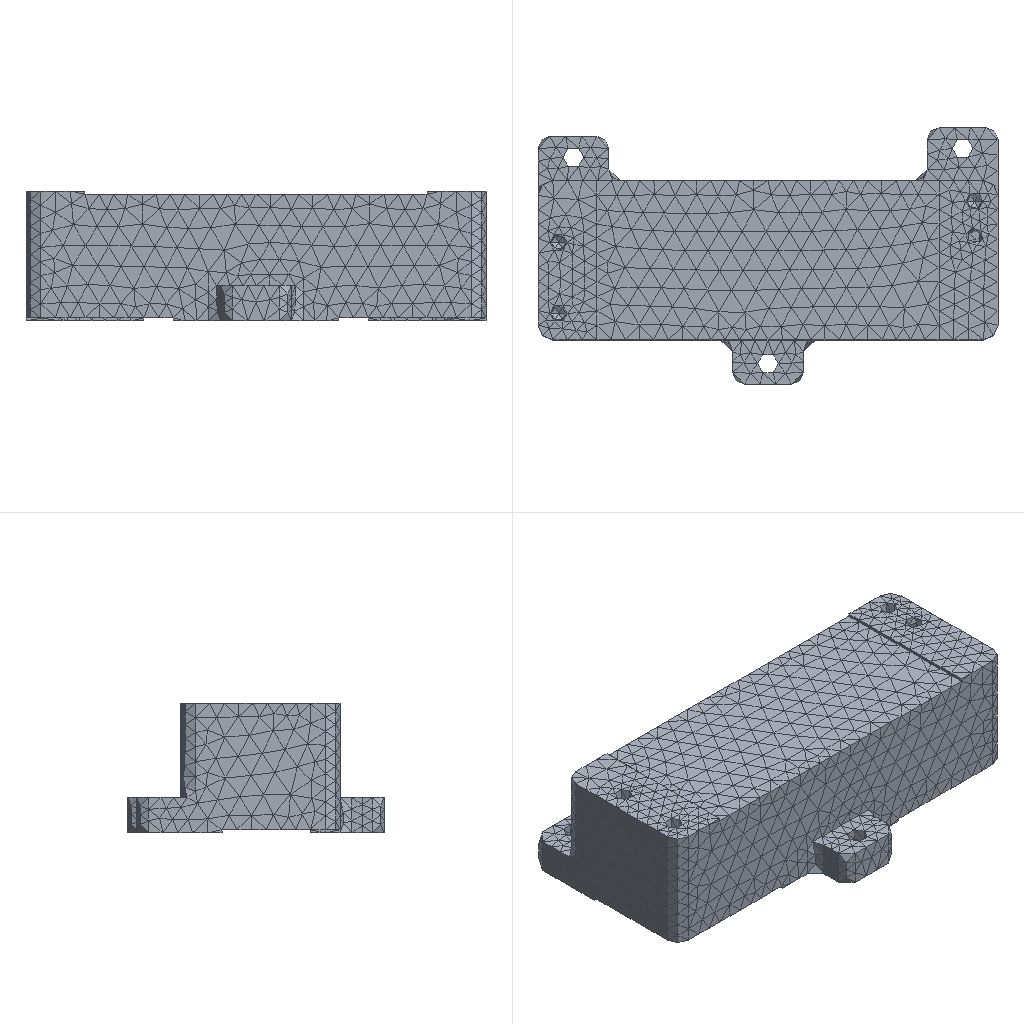Simulation study | nx simcenter
Set-up summary:
category,name,step,type,value,unit,region
solver,nx_nastran (Simcenter)
units,not stated in the deck,,not stated
analysis,deck,,static,static
analysis,solution,,SOL,101
load_step,SUBCASE 1,1,SUBCASE,SPC=1 LOAD=2
load_step,requested,,,1
mesh,nodes,,,12428
mesh,elements,,,6443
element_type,CTETRA,,solid,6443
load,nodal force total,,FX,0.0,model units
load,nodal force total,,FY,0.0,model units
load,nodal force total,,FZ,-2559999.93,model units
load,load commands in deck,,count,390
bc,support commands in deck,,count,578
analysis,NX solution 0,,Structural,Linear Statics - Single Constraint
check,setup vs results,,match,every grid point's frame and coordinates and every element id; grid points of CTETRA elements
Nastran input file, long lists of numbers shortened:
$*$$$$$$$$$$$$$$$$$$$$$$$$$$$$$$$$$$$$$$$$$$$$$$$$$$$$$$$$$$$$$$$$$
$*
$*                    NX v10.0.0.24 TRANSLATOR
$*                    FOR NX NASTRAN VERSION 10.0
$ (33 more lines like these left out)
ASSIGN OUTPUT2='132_sim1-solution_1.op2' UNIT=12
$*
$*$$$$$$$$$$$$$$$$$$$$$$$$$$$$$$$$$$$
$*
$* EXECUTIVE CONTROL
$*
$*$$$$$$$$$$$$$$$$$$$$$$$$$$$$$$$$$$$
$*
ID,NASTRAN,132_sim1-solution_1
SOL 101
CEND
$*
$*$$$$$$$$$$$$$$$$$$$$$$$$$$$$$$$$$$$
$*
$* CASE CONTROL
$*
$*$$$$$$$$$$$$$$$$$$$$$$$$$$$$$$$$$$$
$*
TITLE = Solution 1
ECHO = NONE
SPC = 1
OUTPUT
BCRESULTS(TRACTION,FORCE,PLOT) = ALL
DISPLACEMENT(PLOT) = ALL
ESE(PLOT) = ALL
FORCE(PLOT,CORNER) = ALL
OLOAD(PLOT) = ALL
SPCFORCES(PLOT) = ALL
STRAIN(PLOT,FIBER,CORNER) = ALL
STRESS(PLOT,CORNER) = ALL
$*  NX Step: Subcase - Static Loads 1
SUBCASE 1
LABEL = Subcase - Static Loads 1
LOAD = 2
$*
$*$$$$$$$$$$$$$$$$$$$$$$$$$$$$$$$$$$$
$*
$* BULK DATA
$*
$*$$$$$$$$$$$$$$$$$$$$$$$$$$$$$$$$$$$
$*
BEGIN BULK
$*
$* PARAM CARDS
$*
PARAM      K6ROT100.0000
PARAM     OIBULK     YES
PARAM    OMACHPR     YES
PARAM       POST      -2
PARAM    POSTEXT     YES
PARAM    UNITSYS   MN-MM
$*
$* GRID CARDS
$*
GRID*              12309               00.0000000000E+005.0000000000E+00+
*       1.0000000000E+00               0
GRID*              12310               00.0000000000E+005.0000000000E+00+
*       4.4000000000E+01               0
$ (24852 more lines like these left out)
$*
$* ELEMENT CARDS
$*
$*  NX Mesh Collector: Solid(1)
$*  NX Mesh: 3d_mesh(1)
CTETRA         1       1   12011       1    9732       2     205     206+
+            207     208     209     210
CTETRA         2       1       1       2       3    9732     209     211+
+            212     206     210     213
$ (12882 more lines like these left out)
$*
$* PROPERTY CARDS
$*
$*  NX Property: PSOLID1
PSOLID         1       1       0                           SMECH
$*
$* MATERIAL CARDS
$*
$*  NX Material: Aluminum_5086
MAT1           17.2000+7        0.3300002.6600-62.5000-5
$*
$* LOAD AND CONSTRAINT CARDS
$*
$*  NX Load and Constraint: Fixed(1)
SPC            1    5652  123456  0.0000
SPC            1    5653  123456  0.0000
SPC            1    5654  123456  0.0000
SPC            1    5655  123456  0.0000
$ (574 more lines like these left out)
$*  NX Load and Constraint: Force(1)
FORCE          2   10310       0 7167.78  0.0000  0.0000-1.00000
FORCE          2   10311       0 7315.30  0.0000  0.0000-1.00000
FORCE          2   10312       0 6988.79  0.0000  0.0000-1.00000
FORCE          2   10313       0 4822.47  0.0000  0.0000-1.00000
$ (386 more lines like these left out)
ENDDATA 6c50711c
Results summary:
result,analysis,,,static
result,last_loadstep,,,1
result,primary field,,,displacements
result,max displacement,,,0.006657,model units
result,reaction total,,FX,-0.004791,model units
result,reaction total,,FY,-0.06803,model units
result,reaction total,,FZ,2560001.25,model units
result,NX solution 0,,loadcases,1,mm